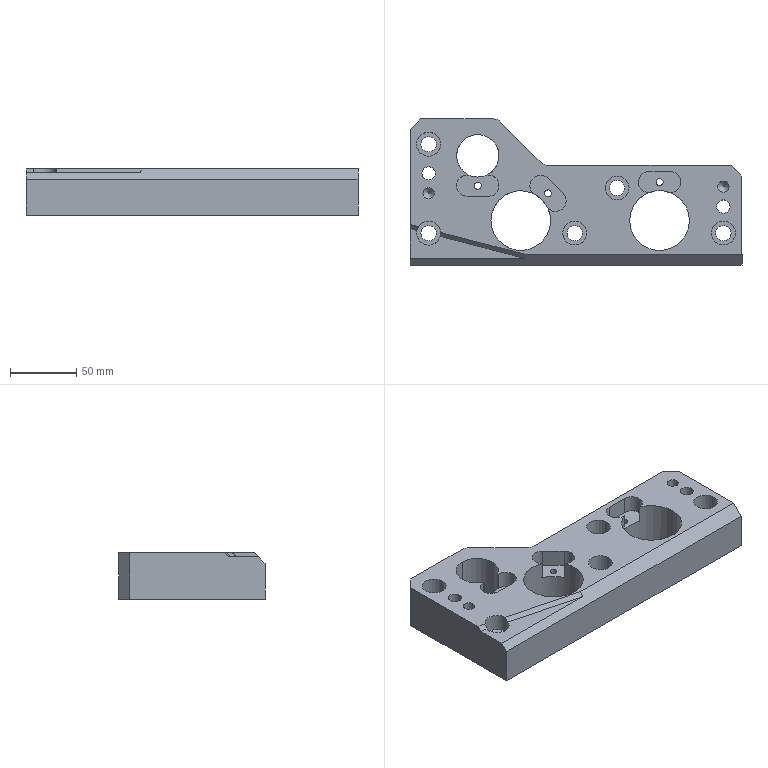Part | STEP file | lll_id4550_x_t | 1 solid | 58 faces | box 250 x 110 x 35 mm | volume 550802 mm3 | cylinder 29 | plane 27 | cone 2 | commonest cylinder face diameters 16 x8 11.509 x5 18.008 x5 5.206 x3 8.506 x2 10 x2